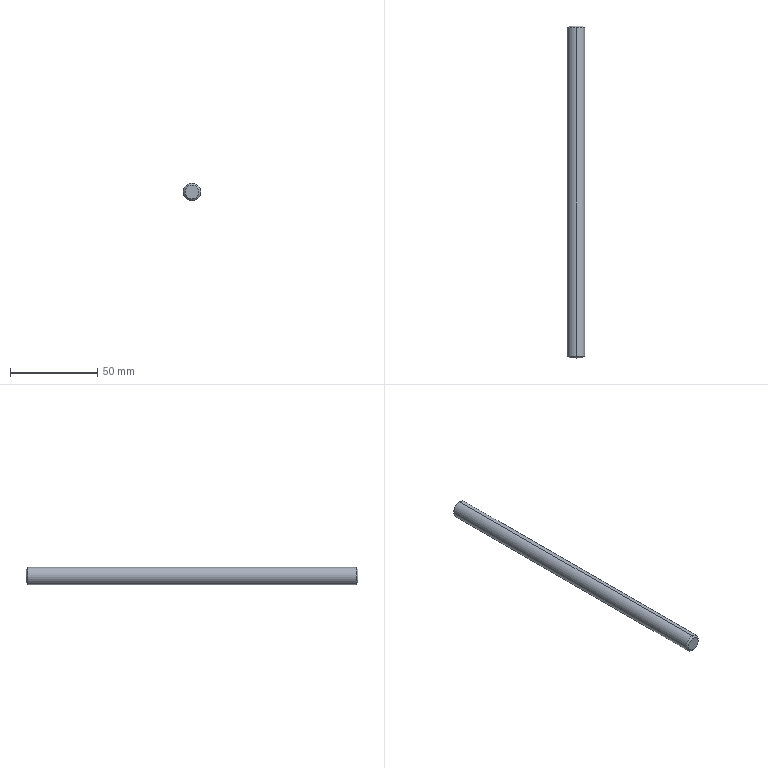Part | STEP file | 1 solid | 8 faces | box 10 x 190 x 10 mm | volume 14893 mm3 | cone 4 | cylinder 2 | plane 2 | commonest cylinder face diameters 10 x2
STEP:
#1=CARTESIAN_POINT('',(0.,0.,0.));
#2=DIRECTION('',(0.,0.,1.));
#3=DIRECTION('',(1.,0.,0.));
#4=AXIS2_PLACEMENT_3D('',#1,#2,#3);
#5=CARTESIAN_POINT('',(0.,0.,-4.));
#6=VERTEX_POINT('',#5);
#7=CARTESIAN_POINT('',(0.,0.,4.));
#8=VERTEX_POINT('',#7);
#9=CARTESIAN_POINT('',(0.,0.,0.));
#10=DIRECTION('',(0.,-1.,0.));
#11=DIRECTION('',(0.,0.,1.));
#12=AXIS2_PLACEMENT_3D('',#9,#10,#11);
#13=CIRCLE('',#12,4.);
#14=CARTESIAN_POINT('',(0.,1.,0.));
#15=DIRECTION('',(0.,1.,0.));
#16=DIRECTION('',(0.,0.,1.));
#17=AXIS2_PLACEMENT_3D('',#14,#15,#16);
#18=CONICAL_SURFACE('',#17,5.,0.7854);
#19=CARTESIAN_POINT('',(6.283,-1.));
#20=DIRECTION('',(-1.,0.));
#21=VECTOR('',#20,1.);
#22=LINE('',#19,#21);
#23=(GEOMETRIC_REPRESENTATION_CONTEXT(2)PARAMETRIC_REPRESENTATION_CONTEXT()REPRESENTATION_CONTEXT('',''));
#24=DEFINITIONAL_REPRESENTATION('',(#22),#23);
#25=PCURVE('',#18,#24);
#26=CARTESIAN_POINT('',(0.,0.,0.));
#27=DIRECTION('',(0.,1.,0.));
#28=DIRECTION('',(0.,0.,1.));
#29=AXIS2_PLACEMENT_3D('',#26,#27,#28);
#30=PLANE('',#29);
#31=CARTESIAN_POINT('',(4.,0.));
#32=CARTESIAN_POINT('',(4.,-6.928));
#33=CARTESIAN_POINT('',(-2.,-3.464));
#34=CARTESIAN_POINT('',(-8.,0.));
#35=CARTESIAN_POINT('',(-2.,3.464));
#36=CARTESIAN_POINT('',(4.,6.928));
#37=CARTESIAN_POINT('',(4.,0.));
#38=(BOUNDED_CURVE()B_SPLINE_CURVE(2,(#31,#32,#33,#34,#35,#36,#37),.UNSPECIFIED.,.T.,.F.)B_SPLINE_CURVE_WITH_KNOTS((1,2,2,2,2,1),(-2.094,0.,2.094,4.189,6.283,8.378),.UNSPECIFIED.)CURVE()GEOMETRIC_REPRESENTATION_ITEM()RATIONAL_B_SPLINE_CURVE((1.,0.5,1.,0.5,1.,0.5,1.))REPRESENTATION_ITEM(''));
#39=(GEOMETRIC_REPRESENTATION_CONTEXT(2)PARAMETRIC_REPRESENTATION_CONTEXT()REPRESENTATION_CONTEXT('',''));
#40=DEFINITIONAL_REPRESENTATION('',(#38),#39);
#41=PCURVE('',#30,#40);
#42=SURFACE_CURVE('',#13,(#25,#41),.PCURVE_S1.);
#43=EDGE_CURVE('',#6,#8,#42,.T.);
#44=ORIENTED_EDGE('',*,*,#43,.F.);
#45=CARTESIAN_POINT('',(0.,1.,-5.));
#46=VERTEX_POINT('',#45);
#47=CARTESIAN_POINT('',(0.,1.,-5.));
#48=DIRECTION('',(0.,0.7071,-0.7071));
#49=VECTOR('',#48,1.);
#50=LINE('',#47,#49);
#51=CARTESIAN_POINT('',(3.142,0.));
#52=DIRECTION('',(0.,1.));
#53=VECTOR('',#52,1.);
#54=LINE('',#51,#53);
#55=(GEOMETRIC_REPRESENTATION_CONTEXT(2)PARAMETRIC_REPRESENTATION_CONTEXT()REPRESENTATION_CONTEXT('',''));
#56=DEFINITIONAL_REPRESENTATION('',(#54),#55);
#57=PCURVE('',#18,#56);
#58=CARTESIAN_POINT('',(0.,1.,0.));
#59=DIRECTION('',(0.,1.,0.));
#60=DIRECTION('',(0.,0.,1.));
#61=AXIS2_PLACEMENT_3D('',#58,#59,#60);
#62=CONICAL_SURFACE('',#61,5.,0.7854);
#63=CARTESIAN_POINT('',(3.142,0.));
#64=DIRECTION('',(0.,1.));
#65=VECTOR('',#64,1.);
#66=LINE('',#63,#65);
#67=(GEOMETRIC_REPRESENTATION_CONTEXT(2)PARAMETRIC_REPRESENTATION_CONTEXT()REPRESENTATION_CONTEXT('',''));
#68=DEFINITIONAL_REPRESENTATION('',(#66),#67);
#69=PCURVE('',#62,#68);
#70=SURFACE_CURVE('',#50,(#57,#69),.PCURVE_S1.);
#71=EDGE_CURVE('',#6,#46,#70,.T.);
#72=ORIENTED_EDGE('',*,*,#71,.T.);
#73=CARTESIAN_POINT('',(0.,1.,5.));
#74=VERTEX_POINT('',#73);
#75=CARTESIAN_POINT('',(0.,1.,0.));
#76=DIRECTION('',(0.,1.,0.));
#77=DIRECTION('',(0.,0.,1.));
#78=AXIS2_PLACEMENT_3D('',#75,#76,#77);
#79=CIRCLE('',#78,5.);
#80=CARTESIAN_POINT('',(0.,0.));
#81=DIRECTION('',(1.,0.));
#82=VECTOR('',#81,1.);
#83=LINE('',#80,#82);
#84=(GEOMETRIC_REPRESENTATION_CONTEXT(2)PARAMETRIC_REPRESENTATION_CONTEXT()REPRESENTATION_CONTEXT('',''));
#85=DEFINITIONAL_REPRESENTATION('',(#83),#84);
#86=PCURVE('',#18,#85);
#87=CARTESIAN_POINT('',(0.,190.,0.));
#88=DIRECTION('',(0.,-1.,0.));
#89=DIRECTION('',(0.,0.,-1.));
#90=AXIS2_PLACEMENT_3D('',#87,#88,#89);
#91=CYLINDRICAL_SURFACE('',#90,5.);
#92=CARTESIAN_POINT('',(3.142,189.));
#93=DIRECTION('',(-1.,0.));
#94=VECTOR('',#93,1.);
#95=LINE('',#92,#94);
#96=(GEOMETRIC_REPRESENTATION_CONTEXT(2)PARAMETRIC_REPRESENTATION_CONTEXT()REPRESENTATION_CONTEXT('',''));
#97=DEFINITIONAL_REPRESENTATION('',(#95),#96);
#98=PCURVE('',#91,#97);
#99=SURFACE_CURVE('',#79,(#86,#98),.PCURVE_S1.);
#100=EDGE_CURVE('',#74,#46,#99,.T.);
#101=ORIENTED_EDGE('',*,*,#100,.F.);
#102=CARTESIAN_POINT('',(0.,1.,5.));
#103=DIRECTION('',(0.,0.7071,0.7071));
#104=VECTOR('',#103,1.);
#105=LINE('',#102,#104);
#106=CARTESIAN_POINT('',(0.,0.));
#107=DIRECTION('',(0.,1.));
#108=VECTOR('',#107,1.);
#109=LINE('',#106,#108);
#110=(GEOMETRIC_REPRESENTATION_CONTEXT(2)PARAMETRIC_REPRESENTATION_CONTEXT()REPRESENTATION_CONTEXT('',''));
#111=DEFINITIONAL_REPRESENTATION('',(#109),#110);
#112=PCURVE('',#18,#111);
#113=CARTESIAN_POINT('',(6.283,0.));
#114=DIRECTION('',(0.,1.));
#115=VECTOR('',#114,1.);
#116=LINE('',#113,#115);
#117=(GEOMETRIC_REPRESENTATION_CONTEXT(2)PARAMETRIC_REPRESENTATION_CONTEXT()REPRESENTATION_CONTEXT('',''));
#118=DEFINITIONAL_REPRESENTATION('',(#116),#117);
#119=PCURVE('',#62,#118);
#120=SURFACE_CURVE('',#105,(#112,#119),.PCURVE_S1.);
#121=EDGE_CURVE('',#8,#74,#120,.T.);
#122=ORIENTED_EDGE('',*,*,#121,.F.);
#123=EDGE_LOOP('',(#44,#72,#101,#122));
#124=FACE_BOUND('',#123,.T.);
#125=ADVANCED_FACE('',(#124),#18,.T.);
#126=CARTESIAN_POINT('',(0.,190.,4.));
#127=VERTEX_POINT('',#126);
#128=CARTESIAN_POINT('',(0.,190.,-4.));
#129=VERTEX_POINT('',#128);
#130=CARTESIAN_POINT('',(0.,190.,0.));
#131=DIRECTION('',(0.,1.,0.));
#132=DIRECTION('',(0.,0.,1.));
#133=AXIS2_PLACEMENT_3D('',#130,#131,#132);
#134=CIRCLE('',#133,4.);
#135=CARTESIAN_POINT('',(0.,190.,0.));
#136=DIRECTION('',(0.,-1.,0.));
#137=DIRECTION('',(0.,0.,-1.));
#138=AXIS2_PLACEMENT_3D('',#135,#136,#137);
#139=CONICAL_SURFACE('',#138,4.,0.7854);
#140=CARTESIAN_POINT('',(3.142,0.));
#141=DIRECTION('',(-1.,0.));
#142=VECTOR('',#141,1.);
#143=LINE('',#140,#142);
#144=(GEOMETRIC_REPRESENTATION_CONTEXT(2)PARAMETRIC_REPRESENTATION_CONTEXT()REPRESENTATION_CONTEXT('',''));
#145=DEFINITIONAL_REPRESENTATION('',(#143),#144);
#146=PCURVE('',#139,#145);
#147=CARTESIAN_POINT('',(0.,190.,0.));
#148=DIRECTION('',(0.,1.,0.));
#149=DIRECTION('',(0.,0.,1.));
#150=AXIS2_PLACEMENT_3D('',#147,#148,#149);
#151=PLANE('',#150);
#152=CARTESIAN_POINT('',(0.,0.));
#153=DIRECTION('',(1.,0.));
#154=AXIS2_PLACEMENT_2D('',#152,#153);
#155=CIRCLE('',#154,4.);
#156=(GEOMETRIC_REPRESENTATION_CONTEXT(2)PARAMETRIC_REPRESENTATION_CONTEXT()REPRESENTATION_CONTEXT('',''));
#157=DEFINITIONAL_REPRESENTATION('',(#155),#156);
#158=PCURVE('',#151,#157);
#159=SURFACE_CURVE('',#134,(#146,#158),.PCURVE_S1.);
#160=EDGE_CURVE('',#127,#129,#159,.T.);
#161=ORIENTED_EDGE('',*,*,#160,.F.);
#162=CARTESIAN_POINT('',(0.,189.,5.));
#163=VERTEX_POINT('',#162);
#164=CARTESIAN_POINT('',(0.,190.,4.));
#165=DIRECTION('',(0.,-0.7071,0.7071));
#166=VECTOR('',#165,1.);
#167=LINE('',#164,#166);
#168=CARTESIAN_POINT('',(3.142,0.));
#169=DIRECTION('',(0.,1.));
#170=VECTOR('',#169,1.);
#171=LINE('',#168,#170);
#172=(GEOMETRIC_REPRESENTATION_CONTEXT(2)PARAMETRIC_REPRESENTATION_CONTEXT()REPRESENTATION_CONTEXT('',''));
#173=DEFINITIONAL_REPRESENTATION('',(#171),#172);
#174=PCURVE('',#139,#173);
#175=CARTESIAN_POINT('',(0.,190.,0.));
#176=DIRECTION('',(0.,-1.,0.));
#177=DIRECTION('',(0.,0.,-1.));
#178=AXIS2_PLACEMENT_3D('',#175,#176,#177);
#179=CONICAL_SURFACE('',#178,4.,0.7854);
#180=CARTESIAN_POINT('',(3.142,0.));
#181=DIRECTION('',(0.,1.));
#182=VECTOR('',#181,1.);
#183=LINE('',#180,#182);
#184=(GEOMETRIC_REPRESENTATION_CONTEXT(2)PARAMETRIC_REPRESENTATION_CONTEXT()REPRESENTATION_CONTEXT('',''));
#185=DEFINITIONAL_REPRESENTATION('',(#183),#184);
#186=PCURVE('',#179,#185);
#187=SURFACE_CURVE('',#167,(#174,#186),.PCURVE_S1.);
#188=EDGE_CURVE('',#127,#163,#187,.T.);
#189=ORIENTED_EDGE('',*,*,#188,.T.);
#190=CARTESIAN_POINT('',(0.,189.,-5.));
#191=VERTEX_POINT('',#190);
#192=CARTESIAN_POINT('',(0.,189.,0.));
#193=DIRECTION('',(0.,-1.,0.));
#194=DIRECTION('',(0.,0.,1.));
#195=AXIS2_PLACEMENT_3D('',#192,#193,#194);
#196=CIRCLE('',#195,5.);
#197=CARTESIAN_POINT('',(-3.142,1.));
#198=DIRECTION('',(1.,0.));
#199=VECTOR('',#198,1.);
#200=LINE('',#197,#199);
#201=(GEOMETRIC_REPRESENTATION_CONTEXT(2)PARAMETRIC_REPRESENTATION_CONTEXT()REPRESENTATION_CONTEXT('',''));
#202=DEFINITIONAL_REPRESENTATION('',(#200),#201);
#203=PCURVE('',#139,#202);
#204=CARTESIAN_POINT('',(-3.142,1.));
#205=DIRECTION('',(1.,0.));
#206=VECTOR('',#205,1.);
#207=LINE('',#204,#206);
#208=(GEOMETRIC_REPRESENTATION_CONTEXT(2)PARAMETRIC_REPRESENTATION_CONTEXT()REPRESENTATION_CONTEXT('',''));
#209=DEFINITIONAL_REPRESENTATION('',(#207),#208);
#210=PCURVE('',#91,#209);
#211=SURFACE_CURVE('',#196,(#203,#210),.PCURVE_S1.);
#212=EDGE_CURVE('',#191,#163,#211,.T.);
#213=ORIENTED_EDGE('',*,*,#212,.F.);
#214=CARTESIAN_POINT('',(0.,190.,-4.));
#215=DIRECTION('',(0.,-0.7071,-0.7071));
#216=VECTOR('',#215,1.);
#217=LINE('',#214,#216);
#218=CARTESIAN_POINT('',(0.,0.));
#219=DIRECTION('',(0.,1.));
#220=VECTOR('',#219,1.);
#221=LINE('',#218,#220);
#222=(GEOMETRIC_REPRESENTATION_CONTEXT(2)PARAMETRIC_REPRESENTATION_CONTEXT()REPRESENTATION_CONTEXT('',''));
#223=DEFINITIONAL_REPRESENTATION('',(#221),#222);
#224=PCURVE('',#139,#223);
#225=CARTESIAN_POINT('',(6.283,0.));
#226=DIRECTION('',(0.,1.));
#227=VECTOR('',#226,1.);
#228=LINE('',#225,#227);
#229=(GEOMETRIC_REPRESENTATION_CONTEXT(2)PARAMETRIC_REPRESENTATION_CONTEXT()REPRESENTATION_CONTEXT('',''));
#230=DEFINITIONAL_REPRESENTATION('',(#228),#229);
#231=PCURVE('',#179,#230);
#232=SURFACE_CURVE('',#217,(#224,#231),.PCURVE_S1.);
#233=EDGE_CURVE('',#129,#191,#232,.T.);
#234=ORIENTED_EDGE('',*,*,#233,.F.);
#235=EDGE_LOOP('',(#161,#189,#213,#234));
#236=FACE_BOUND('',#235,.T.);
#237=ADVANCED_FACE('',(#236),#139,.T.);
#238=ORIENTED_EDGE('',*,*,#212,.T.);
#239=CARTESIAN_POINT('',(0.,190.,5.));
#240=DIRECTION('',(0.,-1.,0.));
#241=VECTOR('',#240,1.);
#242=LINE('',#239,#241);
#243=CARTESIAN_POINT('',(3.142,0.));
#244=DIRECTION('',(0.,1.));
#245=VECTOR('',#244,1.);
#246=LINE('',#243,#245);
#247=(GEOMETRIC_REPRESENTATION_CONTEXT(2)PARAMETRIC_REPRESENTATION_CONTEXT()REPRESENTATION_CONTEXT('',''));
#248=DEFINITIONAL_REPRESENTATION('',(#246),#247);
#249=PCURVE('',#91,#248);
#250=CARTESIAN_POINT('',(0.,190.,0.));
#251=DIRECTION('',(0.,-1.,0.));
#252=DIRECTION('',(0.,0.,-1.));
#253=AXIS2_PLACEMENT_3D('',#250,#251,#252);
#254=CYLINDRICAL_SURFACE('',#253,5.);
#255=CARTESIAN_POINT('',(3.142,0.));
#256=DIRECTION('',(0.,1.));
#257=VECTOR('',#256,1.);
#258=LINE('',#255,#257);
#259=(GEOMETRIC_REPRESENTATION_CONTEXT(2)PARAMETRIC_REPRESENTATION_CONTEXT()REPRESENTATION_CONTEXT('',''));
#260=DEFINITIONAL_REPRESENTATION('',(#258),#259);
#261=PCURVE('',#254,#260);
#262=SURFACE_CURVE('',#242,(#249,#261),.PCURVE_S1.);
#263=EDGE_CURVE('',#163,#74,#262,.T.);
#264=ORIENTED_EDGE('',*,*,#263,.T.);
#265=ORIENTED_EDGE('',*,*,#100,.T.);
#266=CARTESIAN_POINT('',(0.,190.,-5.));
#267=DIRECTION('',(0.,-1.,0.));
#268=VECTOR('',#267,1.);
#269=LINE('',#266,#268);
#270=CARTESIAN_POINT('',(0.,0.));
#271=DIRECTION('',(0.,1.));
#272=VECTOR('',#271,1.);
#273=LINE('',#270,#272);
#274=(GEOMETRIC_REPRESENTATION_CONTEXT(2)PARAMETRIC_REPRESENTATION_CONTEXT()REPRESENTATION_CONTEXT('',''));
#275=DEFINITIONAL_REPRESENTATION('',(#273),#274);
#276=PCURVE('',#91,#275);
#277=CARTESIAN_POINT('',(6.283,0.));
#278=DIRECTION('',(0.,1.));
#279=VECTOR('',#278,1.);
#280=LINE('',#277,#279);
#281=(GEOMETRIC_REPRESENTATION_CONTEXT(2)PARAMETRIC_REPRESENTATION_CONTEXT()REPRESENTATION_CONTEXT('',''));
#282=DEFINITIONAL_REPRESENTATION('',(#280),#281);
#283=PCURVE('',#254,#282);
#284=SURFACE_CURVE('',#269,(#276,#283),.PCURVE_S1.);
#285=EDGE_CURVE('',#191,#46,#284,.T.);
#286=ORIENTED_EDGE('',*,*,#285,.F.);
#287=EDGE_LOOP('',(#238,#264,#265,#286));
#288=FACE_BOUND('',#287,.T.);
#289=ADVANCED_FACE('',(#288),#91,.T.);
#290=ORIENTED_EDGE('',*,*,#263,.F.);
#291=CARTESIAN_POINT('',(0.,189.,0.));
#292=DIRECTION('',(0.,-1.,0.));
#293=DIRECTION('',(0.,0.,1.));
#294=AXIS2_PLACEMENT_3D('',#291,#292,#293);
#295=CIRCLE('',#294,5.);
#296=CARTESIAN_POINT('',(3.142,1.));
#297=DIRECTION('',(1.,0.));
#298=VECTOR('',#297,1.);
#299=LINE('',#296,#298);
#300=(GEOMETRIC_REPRESENTATION_CONTEXT(2)PARAMETRIC_REPRESENTATION_CONTEXT()REPRESENTATION_CONTEXT('',''));
#301=DEFINITIONAL_REPRESENTATION('',(#299),#300);
#302=PCURVE('',#254,#301);
#303=CARTESIAN_POINT('',(3.142,1.));
#304=DIRECTION('',(1.,0.));
#305=VECTOR('',#304,1.);
#306=LINE('',#303,#305);
#307=(GEOMETRIC_REPRESENTATION_CONTEXT(2)PARAMETRIC_REPRESENTATION_CONTEXT()REPRESENTATION_CONTEXT('',''));
#308=DEFINITIONAL_REPRESENTATION('',(#306),#307);
#309=PCURVE('',#179,#308);
#310=SURFACE_CURVE('',#295,(#302,#309),.PCURVE_S1.);
#311=EDGE_CURVE('',#163,#191,#310,.T.);
#312=ORIENTED_EDGE('',*,*,#311,.T.);
#313=ORIENTED_EDGE('',*,*,#285,.T.);
#314=CARTESIAN_POINT('',(0.,1.,0.));
#315=DIRECTION('',(0.,1.,0.));
#316=DIRECTION('',(0.,0.,1.));
#317=AXIS2_PLACEMENT_3D('',#314,#315,#316);
#318=CIRCLE('',#317,5.);
#319=CARTESIAN_POINT('',(9.425,189.));
#320=DIRECTION('',(-1.,0.));
#321=VECTOR('',#320,1.);
#322=LINE('',#319,#321);
#323=(GEOMETRIC_REPRESENTATION_CONTEXT(2)PARAMETRIC_REPRESENTATION_CONTEXT()REPRESENTATION_CONTEXT('',''));
#324=DEFINITIONAL_REPRESENTATION('',(#322),#323);
#325=PCURVE('',#254,#324);
#326=CARTESIAN_POINT('',(0.,0.));
#327=DIRECTION('',(1.,0.));
#328=VECTOR('',#327,1.);
#329=LINE('',#326,#328);
#330=(GEOMETRIC_REPRESENTATION_CONTEXT(2)PARAMETRIC_REPRESENTATION_CONTEXT()REPRESENTATION_CONTEXT('',''));
#331=DEFINITIONAL_REPRESENTATION('',(#329),#330);
#332=PCURVE('',#62,#331);
#333=SURFACE_CURVE('',#318,(#325,#332),.PCURVE_S1.);
#334=EDGE_CURVE('',#46,#74,#333,.T.);
#335=ORIENTED_EDGE('',*,*,#334,.T.);
#336=EDGE_LOOP('',(#290,#312,#313,#335));
#337=FACE_BOUND('',#336,.T.);
#338=ADVANCED_FACE('',(#337),#254,.T.);
#339=CARTESIAN_POINT('',(0.,190.,0.));
#340=DIRECTION('',(0.,1.,0.));
#341=DIRECTION('',(0.,0.,1.));
#342=AXIS2_PLACEMENT_3D('',#339,#340,#341);
#343=CIRCLE('',#342,4.);
#344=CARTESIAN_POINT('',(0.,0.));
#345=DIRECTION('',(1.,0.));
#346=AXIS2_PLACEMENT_2D('',#344,#345);
#347=CIRCLE('',#346,4.);
#348=(GEOMETRIC_REPRESENTATION_CONTEXT(2)PARAMETRIC_REPRESENTATION_CONTEXT()REPRESENTATION_CONTEXT('',''));
#349=DEFINITIONAL_REPRESENTATION('',(#347),#348);
#350=PCURVE('',#151,#349);
#351=CARTESIAN_POINT('',(9.425,0.));
#352=DIRECTION('',(-1.,0.));
#353=VECTOR('',#352,1.);
#354=LINE('',#351,#353);
#355=(GEOMETRIC_REPRESENTATION_CONTEXT(2)PARAMETRIC_REPRESENTATION_CONTEXT()REPRESENTATION_CONTEXT('',''));
#356=DEFINITIONAL_REPRESENTATION('',(#354),#355);
#357=PCURVE('',#179,#356);
#358=SURFACE_CURVE('',#343,(#350,#357),.PCURVE_S1.);
#359=EDGE_CURVE('',#129,#127,#358,.T.);
#360=ORIENTED_EDGE('',*,*,#359,.T.);
#361=ORIENTED_EDGE('',*,*,#160,.T.);
#362=EDGE_LOOP('',(#360,#361));
#363=FACE_BOUND('',#362,.T.);
#364=ADVANCED_FACE('',(#363),#151,.T.);
#365=CARTESIAN_POINT('',(0.,0.,0.));
#366=DIRECTION('',(0.,-1.,0.));
#367=DIRECTION('',(0.,0.,1.));
#368=AXIS2_PLACEMENT_3D('',#365,#366,#367);
#369=CIRCLE('',#368,4.);
#370=CARTESIAN_POINT('',(4.,0.));
#371=CARTESIAN_POINT('',(4.,-6.928));
#372=CARTESIAN_POINT('',(-2.,-3.464));
#373=CARTESIAN_POINT('',(-8.,0.));
#374=CARTESIAN_POINT('',(-2.,3.464));
#375=CARTESIAN_POINT('',(4.,6.928));
#376=CARTESIAN_POINT('',(4.,0.));
#377=(BOUNDED_CURVE()B_SPLINE_CURVE(2,(#370,#371,#372,#373,#374,#375,#376),.UNSPECIFIED.,.T.,.F.)B_SPLINE_CURVE_WITH_KNOTS((1,2,2,2,2,1),(-2.094,0.,2.094,4.189,6.283,8.378),.UNSPECIFIED.)CURVE()GEOMETRIC_REPRESENTATION_ITEM()RATIONAL_B_SPLINE_CURVE((1.,0.5,1.,0.5,1.,0.5,1.))REPRESENTATION_ITEM(''));
#378=(GEOMETRIC_REPRESENTATION_CONTEXT(2)PARAMETRIC_REPRESENTATION_CONTEXT()REPRESENTATION_CONTEXT('',''));
#379=DEFINITIONAL_REPRESENTATION('',(#377),#378);
#380=PCURVE('',#30,#379);
#381=CARTESIAN_POINT('',(6.283,-1.));
#382=DIRECTION('',(-1.,0.));
#383=VECTOR('',#382,1.);
#384=LINE('',#381,#383);
#385=(GEOMETRIC_REPRESENTATION_CONTEXT(2)PARAMETRIC_REPRESENTATION_CONTEXT()REPRESENTATION_CONTEXT('',''));
#386=DEFINITIONAL_REPRESENTATION('',(#384),#385);
#387=PCURVE('',#62,#386);
#388=SURFACE_CURVE('',#369,(#380,#387),.PCURVE_S1.);
#389=EDGE_CURVE('',#8,#6,#388,.T.);
#390=ORIENTED_EDGE('',*,*,#389,.T.);
#391=ORIENTED_EDGE('',*,*,#43,.T.);
#392=EDGE_LOOP('',(#390,#391));
#393=FACE_BOUND('',#392,.T.);
#394=ADVANCED_FACE('',(#393),#30,.F.);
#395=ORIENTED_EDGE('',*,*,#188,.F.);
#396=ORIENTED_EDGE('',*,*,#359,.F.);
#397=ORIENTED_EDGE('',*,*,#233,.T.);
#398=ORIENTED_EDGE('',*,*,#311,.F.);
#399=EDGE_LOOP('',(#395,#396,#397,#398));
#400=FACE_BOUND('',#399,.T.);
#401=ADVANCED_FACE('',(#400),#179,.T.);
#402=ORIENTED_EDGE('',*,*,#71,.F.);
#403=ORIENTED_EDGE('',*,*,#389,.F.);
#404=ORIENTED_EDGE('',*,*,#121,.T.);
#405=ORIENTED_EDGE('',*,*,#334,.F.);
#406=EDGE_LOOP('',(#402,#403,#404,#405));
#407=FACE_BOUND('',#406,.T.);
#408=ADVANCED_FACE('',(#407),#62,.T.);
#409=CLOSED_SHELL('',(#125,#237,#289,#338,#364,#394,#401,#408));
#410=MANIFOLD_SOLID_BREP('',#409);
#411=(LENGTH_UNIT()NAMED_UNIT(*)SI_UNIT(.MILLI.,.METRE.));
#412=UNCERTAINTY_MEASURE_WITH_UNIT(LENGTH_MEASURE(0.0000001),#411,'','');
#413=(NAMED_UNIT(*)PLANE_ANGLE_UNIT()SI_UNIT($,.RADIAN.));
#414=(NAMED_UNIT(*)SI_UNIT($,.STERADIAN.)SOLID_ANGLE_UNIT());
#415=(GEOMETRIC_REPRESENTATION_CONTEXT(3)GLOBAL_UNCERTAINTY_ASSIGNED_CONTEXT((#412))GLOBAL_UNIT_ASSIGNED_CONTEXT((#411,#413,#414))REPRESENTATION_CONTEXT('',''));
#416=ADVANCED_BREP_SHAPE_REPRESENTATION('',(#4,#410),#415);